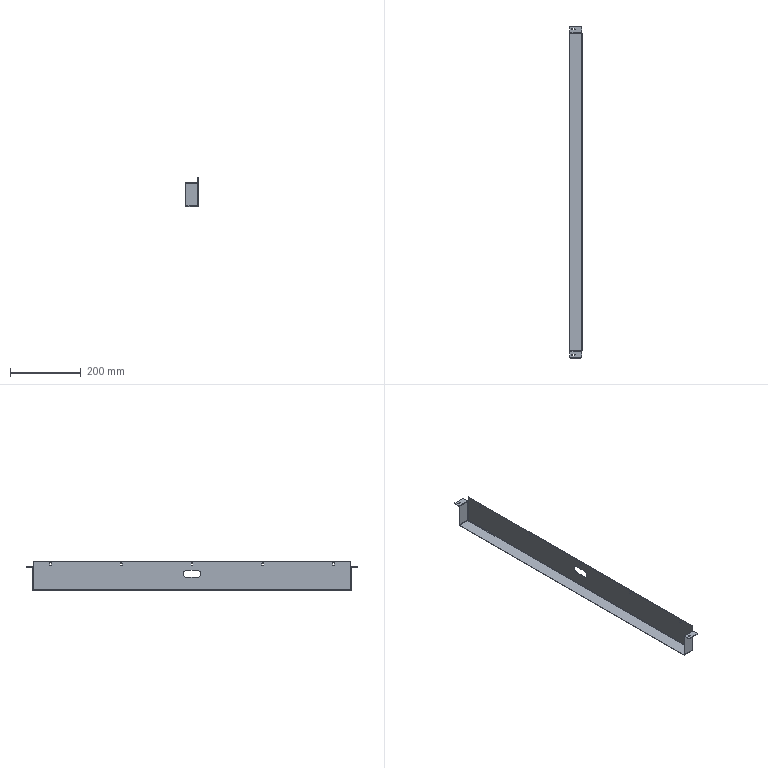Part | SolidWorks | features BaseBody 1 | 1 solid | 91 faces | box 35 x 938 x 82 mm | volume 107925 mm3 | plane 48 | cylinder 39 | spline 4 | commonest cylinder face diameters 4.5 x21 4 x11 2 x5 20 x2